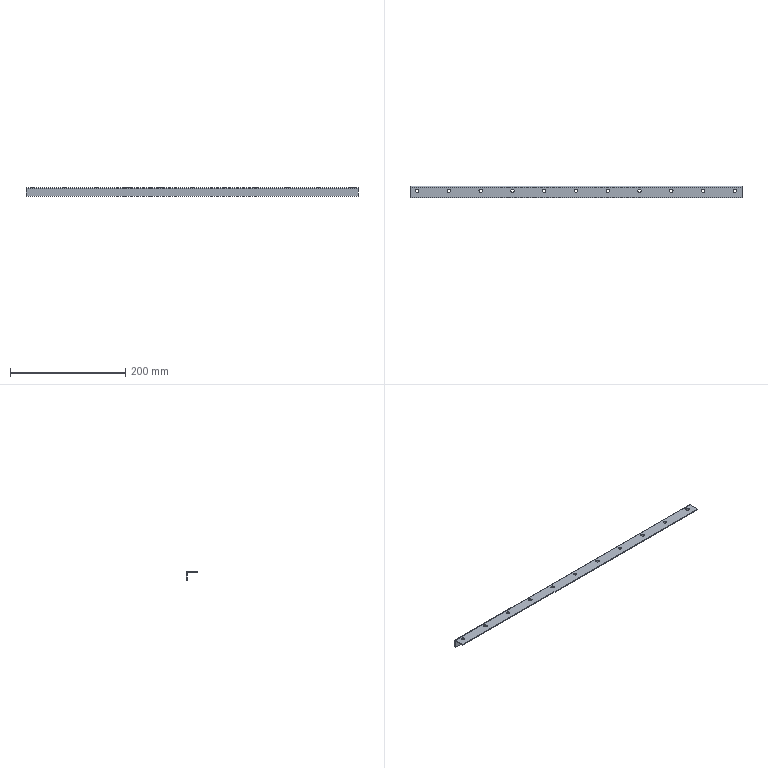Part | STEP file | FHD-021-001-W rack welded part W | 1 solid | 21 faces | box 575 x 20 x 15 mm | volume 28039 mm3 | cylinder 13 | plane 8 | commonest cylinder face diameters 6 x11 0.6 x1 3.6 x1